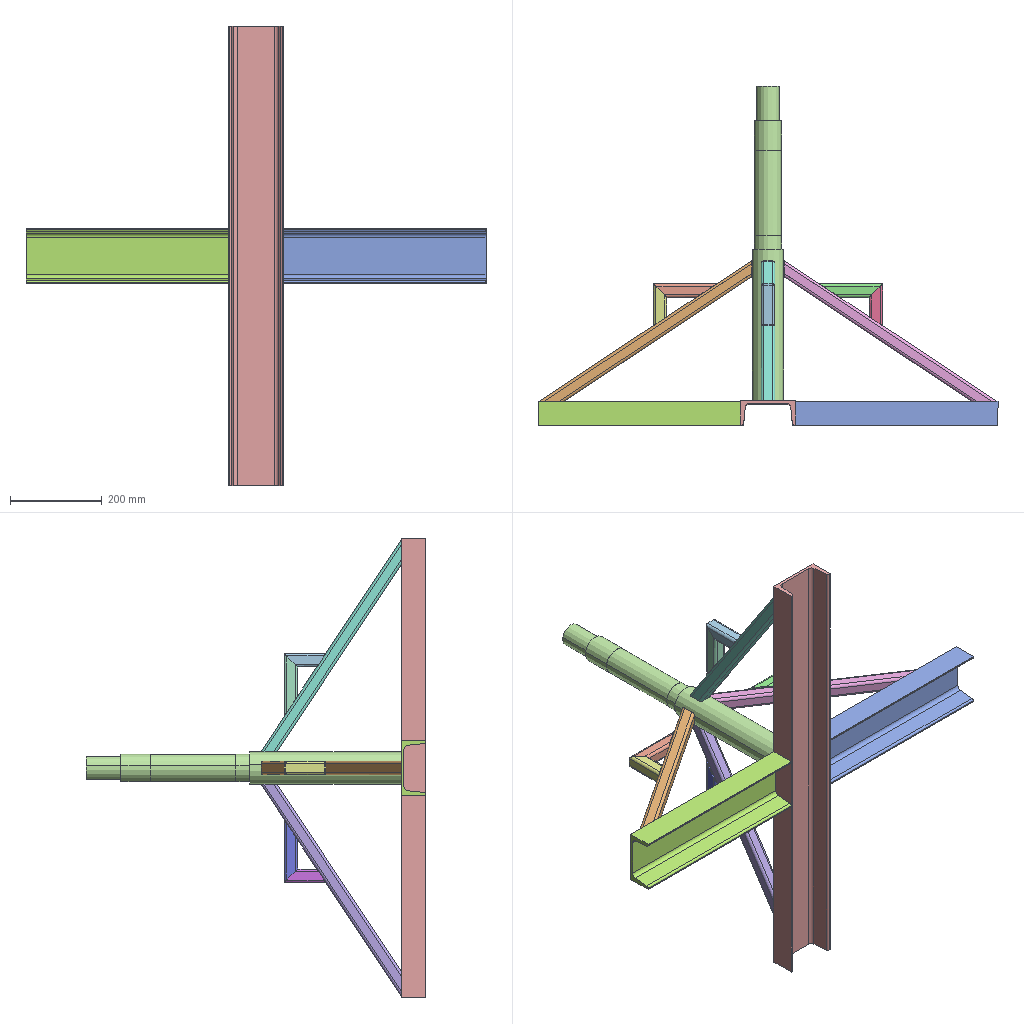Assembly | SolidWorks | 9 different items | 10 placed | box 1000 x 738 x 1000 mm
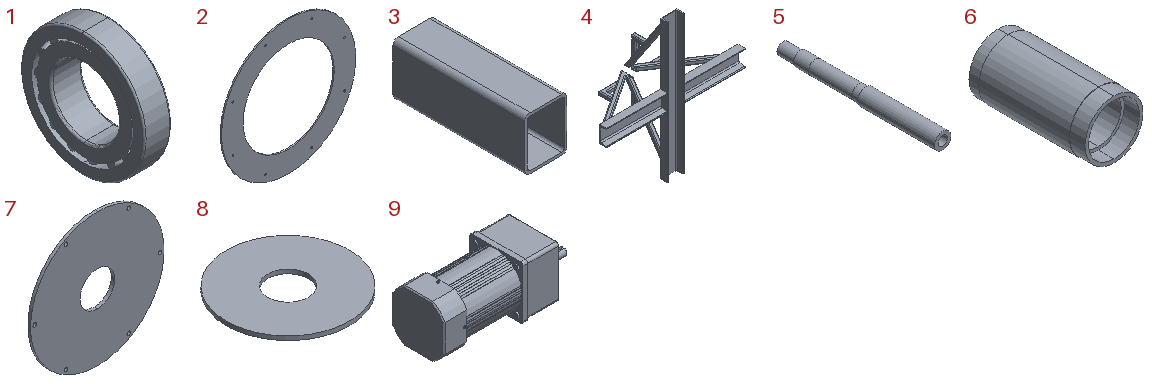Parts list (item | quantity | size | volume | features):
1 | x2 | 29.75 x 110 x 110 mm | 136035 mm3 | features Revolution 3, Fillet 2, CirPattern 1, RefAxis 1
2 | x1 | 1000 x 10 x 1000 mm | 4210849 mm3 | features Extrusion 1, HoleWzd 1
3 | x1 | 80 x 250 x 100 mm | 408905 mm3 | features WeldMemberFeat 1, WeldmentFeature 1
4 | x1 | 1000 x 358.035 x 1000 mm | 3764045 mm3 | features WeldMemberFeat 3, WeldCornerFeat 2, CirPattern 1, ICE 1, RefAxis 1, WeldmentFeature 1
5 | x1 | 70 x 685 x 70 mm | 1330845 mm3 | features ICE 1, Revolution 1
6 | x1 | 127 x 250 x 127 mm | 1158206 mm3 | features Revolution 1
7 | x1 | 480 x 12 x 480 mm | 1930239 mm3 | features Extrusion 1, HoleWzd 1, ICE 1
8 | x1 | 380 x 380 x 12.5 mm | 1263016 mm3 | features Extrusion 1
9 | x1 | 277 x 108.652 x 108.652 mm | 2249960 mm3 | features ICE 13, Fillet 4, Chamfer 3, CirPattern 3, Revolution 2, Extrusion 1, LibraryFeature 1, MoveFace 1
Mates (type | each side: item.copy, entity, surface, feature):
Coincident | 4.1 plane | assembly plane | 2 times
Coincident | 4.1 face plane Gb/t 707—1988 hot-rolled plain channel 120X53X5.5 type 12#-example.com(1) | 5.1 face plane Revolve1
Concentric | 6.1 face cylinder Revolve1 | 1.1 face cylinder Base-Revolve
Coincident | 6.1 face plane Revolve1 | 1.1 face plane Boss-Revolve16
Concentric | 6.1 face cylinder Revolve1 | 1.2 face cylinder Base-Revolve
Coincident | 6.1 face plane Revolve1 | 1.2 face plane Boss-Revolve16
Concentric | 6.1 face cylinder Revolve1 | 7.1 face cylinder Boss-Extrude1
Coincident | 6.1 face plane Revolve1 | 7.1 face plane Boss-Extrude1
Concentric | 6.1 face cylinder Revolve1 | 8.1 face cylinder Boss-Extrude1
Coincident | 6.1 face plane Revolve1 | 8.1 face plane Boss-Extrude1
Coincident | 1.1 face plane Base-Revolve | 5.1 face plane Revolve1
Concentric | 6.1 face cylinder Revolve1 | 5.1 face cylinder Revolve1
DistanceDim | 9.1 face cylinder Revolve2 | 7.1 face cylinder Boss-Extrude1
Coincident | 2.1 face plane Boss-Extrude1 | 3.1 face plane Gb/t 6728—2002 rectangular hollow section 100X80X5(1)
Concentric | 2.1 face cylinder Boss-Extrude1 | 6.1 face cylinder Revolve1